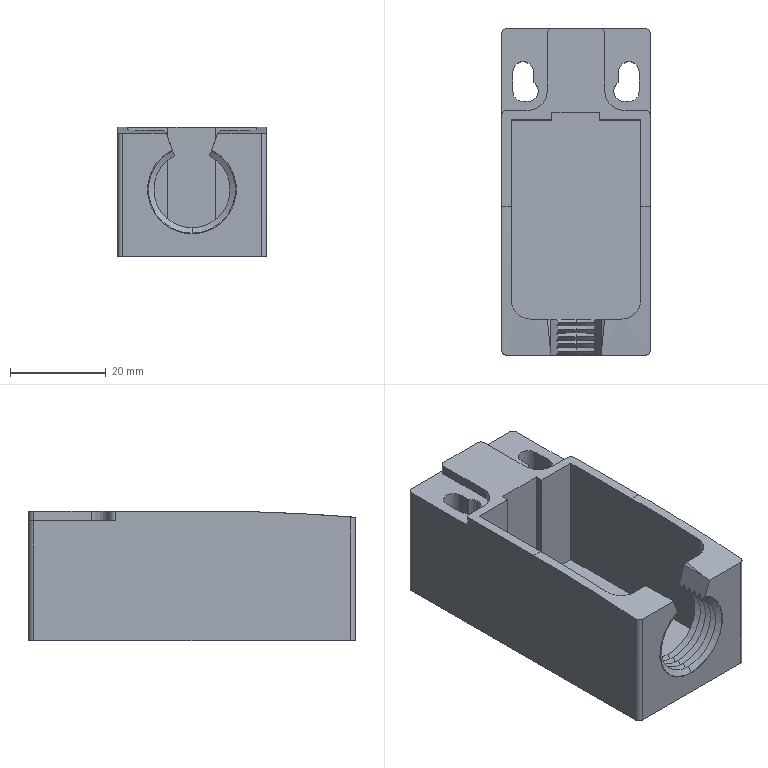Part | STEP file | 2023_07_21_12_39_19_0144 | 1 solid | 113 faces | box 31 x 68 x 27 mm | volume 22352 mm3 | plane 63 | cylinder 28 | cone 22 | commonest cylinder face diameters 2 x8 4.3 x6 1 x2 4 x2 7 x2 7.82 x2